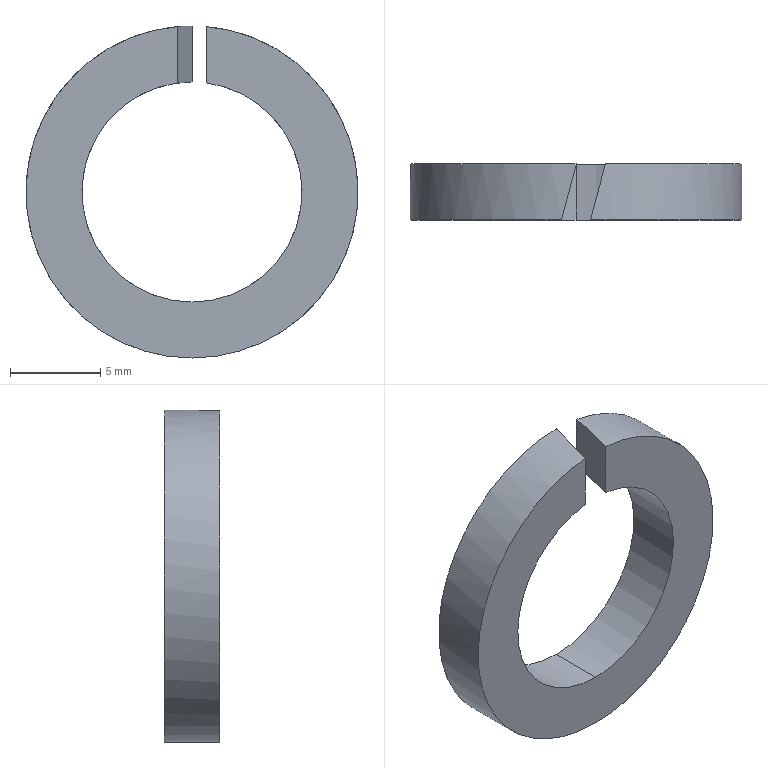Part | SolidWorks | features ICE 2, Extrusion 1 | 1 solid | 482 faces | box 18.4 x 3.1 x 18.4 mm | volume 446.274 mm3 | plane 337 | spline 139 | cylinder 6 | commonest cylinder face diameters 12.2 x3 18.4 x3